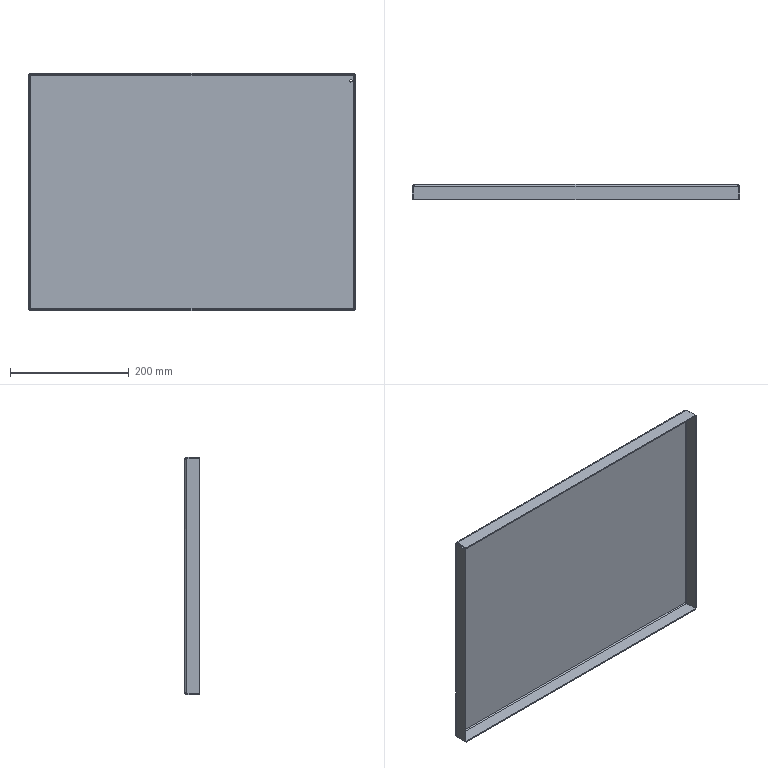Part | SolidWorks | features Cut 1, EdgeFlange 1, FlatPattern 1, SMBaseFlange 1, SheetMetal 1 | 1 solid | 40 faces | box 550 x 25 x 400 mm | volume 521630 mm3 | plane 22 | cylinder 10 | spline 8 | commonest cylinder face diameters 4 x4 8 x4 4.2 x2